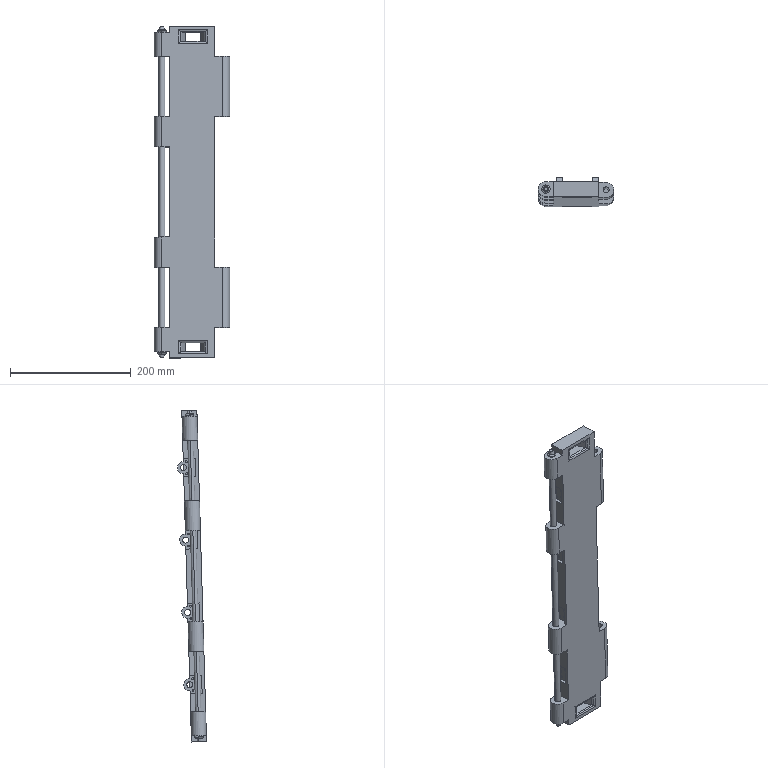Part | SolidWorks | 4 solids | 236 faces | box 125 x 48.263 x 550.495 mm | volume 785015 mm3 | cylinder 108 | plane 104 | torus 20 | cone 4 | commonest cylinder face diameters 3 x32 10 x30 8 x16 12 x16 20 x8 25 x6